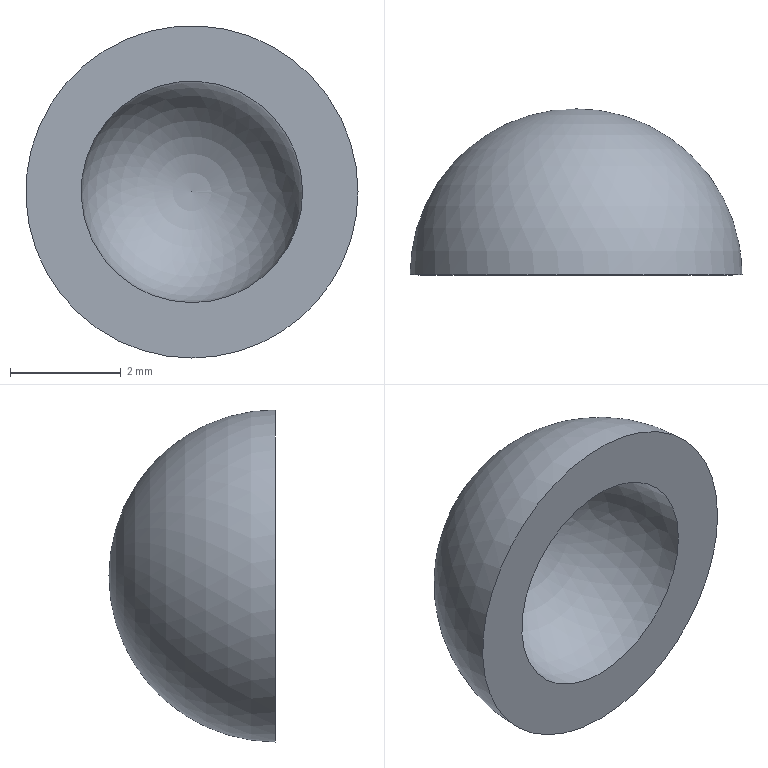Part | NX | features DATUM_CSYS 2, SHELL 1, SKETCH 1, SWP104 1 | 1 solid | 3 faces | box 6 x 3 x 6 mm | volume 39.794 mm3 | sphere 2 | plane 1
STEP:
#1=CARTESIAN_POINT('',(0.,0.,-2.));
#2=VERTEX_POINT('',#1);
#3=CARTESIAN_POINT('',(0.,0.,0.));
#4=DIRECTION('',(0.,-1.,0.));
#5=DIRECTION('',(0.,0.,-1.));
#6=AXIS2_PLACEMENT_3D('',#3,#4,#5);
#7=CIRCLE('',#6,2.);
#8=EDGE_CURVE('',#2,#2,#7,.T.);
#9=ORIENTED_EDGE('',*,*,#8,.F.);
#10=EDGE_LOOP('',(#9));
#11=FACE_BOUND('',#10,.T.);
#12=CARTESIAN_POINT('',(0.,0.,-3.));
#13=VERTEX_POINT('',#12);
#14=CARTESIAN_POINT('',(0.,0.,0.));
#15=DIRECTION('',(0.,-1.,0.));
#16=DIRECTION('',(0.,0.,-1.));
#17=AXIS2_PLACEMENT_3D('',#14,#15,#16);
#18=CIRCLE('',#17,3.);
#19=EDGE_CURVE('',#13,#13,#18,.T.);
#20=ORIENTED_EDGE('',*,*,#19,.T.);
#21=EDGE_LOOP('',(#20));
#22=FACE_BOUND('',#21,.T.);
#23=CARTESIAN_POINT('',(0.,0.,0.));
#24=DIRECTION('',(0.,-1.,0.));
#25=DIRECTION('',(0.,0.,-1.));
#26=AXIS2_PLACEMENT_3D('',#23,#24,#25);
#27=PLANE('',#26);
#28=ADVANCED_FACE('',(#11,#22),#27,.T.);
#29=ORIENTED_EDGE('',*,*,#19,.F.);
#30=EDGE_LOOP('',(#29));
#31=FACE_BOUND('',#30,.T.);
#32=CARTESIAN_POINT('',(0.,0.,0.));
#33=DIRECTION('',(0.,-1.,0.));
#34=DIRECTION('',(1.,0.,0.));
#35=AXIS2_PLACEMENT_3D('',#32,#33,#34);
#36=SPHERICAL_SURFACE('',#35,3.);
#37=ADVANCED_FACE('',(#31),#36,.T.);
#38=ORIENTED_EDGE('',*,*,#8,.T.);
#39=EDGE_LOOP('',(#38));
#40=FACE_BOUND('',#39,.T.);
#41=CARTESIAN_POINT('',(0.,0.,0.));
#42=DIRECTION('',(0.,-1.,0.));
#43=DIRECTION('',(1.,0.,0.));
#44=AXIS2_PLACEMENT_3D('',#41,#42,#43);
#45=SPHERICAL_SURFACE('',#44,2.);
#46=ADVANCED_FACE('',(#40),#45,.F.);
#47=CLOSED_SHELL('',(#28,#37,#46));
#48=MANIFOLD_SOLID_BREP('',#47);
#49=(LENGTH_UNIT()NAMED_UNIT(*)SI_UNIT(.MILLI.,.METRE.));
#50=UNCERTAINTY_MEASURE_WITH_UNIT(LENGTH_MEASURE(0.00001),#49,'','');
#51=(NAMED_UNIT(*)PLANE_ANGLE_UNIT()SI_UNIT($,.RADIAN.));
#52=(NAMED_UNIT(*)SI_UNIT($,.STERADIAN.)SOLID_ANGLE_UNIT());
#53=(GEOMETRIC_REPRESENTATION_CONTEXT(3)GLOBAL_UNCERTAINTY_ASSIGNED_CONTEXT((#50))GLOBAL_UNIT_ASSIGNED_CONTEXT((#49,#51,#52))REPRESENTATION_CONTEXT('',''));
#54=ADVANCED_BREP_SHAPE_REPRESENTATION('',(#48),#53);